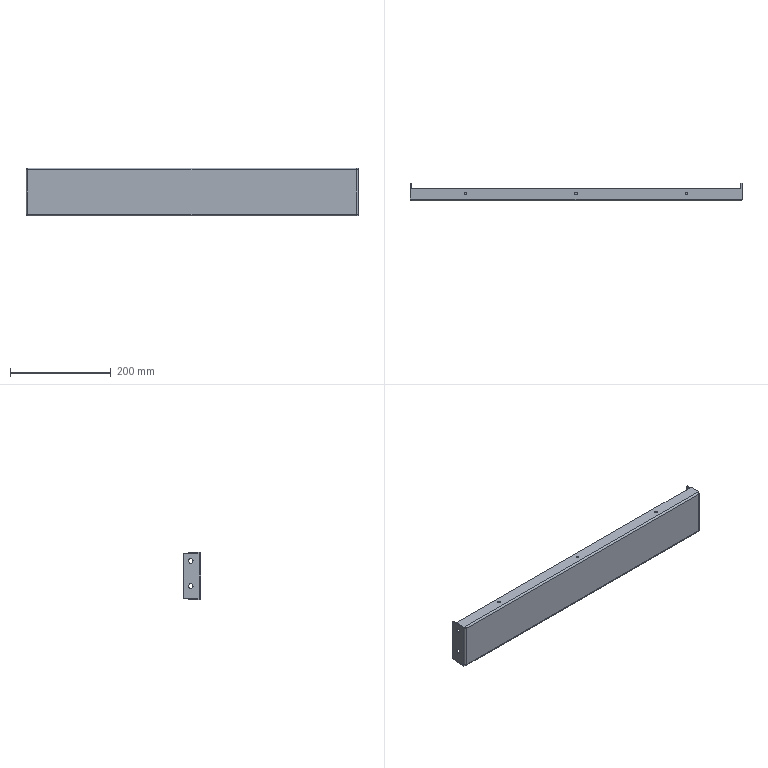Part | STEP file | 5.11.8.01.0013.1 DoorBeam | 1 solid | 60 faces | box 660 x 35 x 95 mm | volume 194127 mm3 | plane 38 | cylinder 22 | commonest cylinder face diameters 9 x8 5.3 x6 3 x4 7 x4